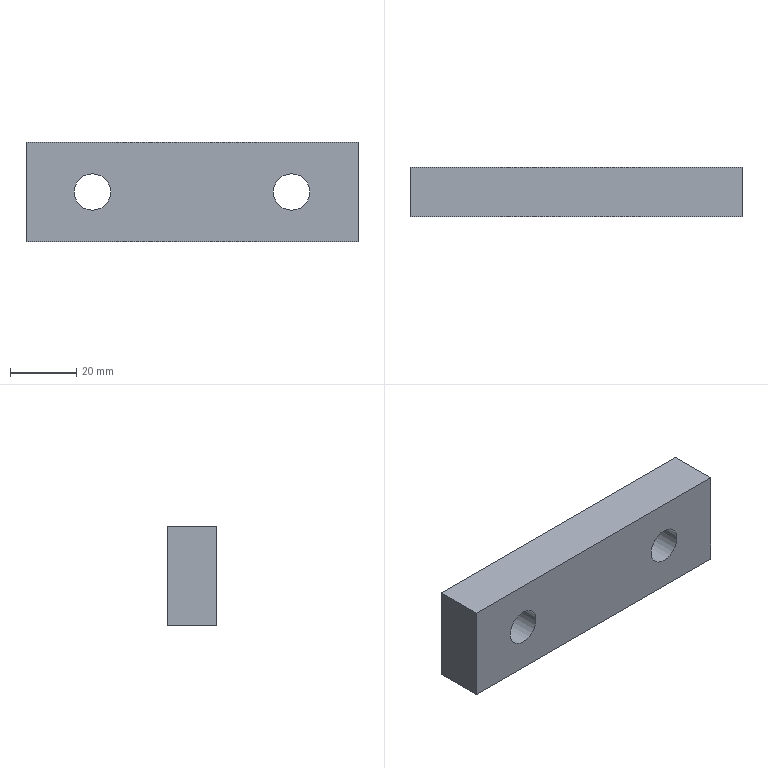Part | STEP file | solid 84 | 1 solid | 8 faces | box 100 x 15 x 30 mm | volume 42149 mm3 | plane 6 | cylinder 2 | commonest cylinder face diameters 11 x2